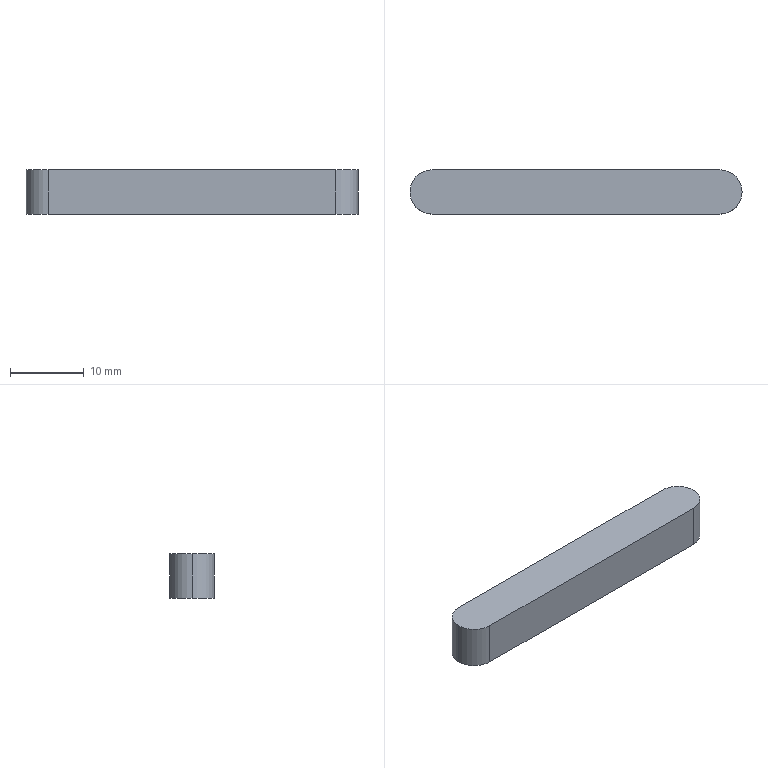Part | STEP file | BPSP-03-008 Flat Key_Default | 1 solid | 8 faces | box 45 x 6 x 6 mm | volume 1574 mm3 | plane 4 | cylinder 4 | commonest cylinder face diameters 6 x4
STEP:
#1=CARTESIAN_POINT('',(0.,0.,0.));
#2=DIRECTION('',(0.,0.,1.));
#3=DIRECTION('',(1.,0.,0.));
#4=AXIS2_PLACEMENT_3D('',#1,#2,#3);
#5=CARTESIAN_POINT('',(19.5,3.,-3.));
#6=VERTEX_POINT('',#5);
#7=CARTESIAN_POINT('',(-19.5,3.,-3.));
#8=VERTEX_POINT('',#7);
#9=CARTESIAN_POINT('',(-22.5,3.,-3.));
#10=DIRECTION('',(-1.,0.,0.));
#11=VECTOR('',#10,1.);
#12=LINE('',#9,#11);
#13=CARTESIAN_POINT('',(-22.5,3.,3.));
#14=DIRECTION('',(0.,-1.,0.));
#15=DIRECTION('',(0.,0.,-1.));
#16=AXIS2_PLACEMENT_3D('',#13,#14,#15);
#17=PLANE('',#16);
#18=CARTESIAN_POINT('',(6.,0.));
#19=DIRECTION('',(0.,-1.));
#20=VECTOR('',#19,1.);
#21=LINE('',#18,#20);
#22=(GEOMETRIC_REPRESENTATION_CONTEXT(2)PARAMETRIC_REPRESENTATION_CONTEXT()REPRESENTATION_CONTEXT('',''));
#23=DEFINITIONAL_REPRESENTATION('',(#21),#22);
#24=PCURVE('',#17,#23);
#25=CARTESIAN_POINT('',(0.,0.,-3.));
#26=DIRECTION('',(0.,0.,1.));
#27=DIRECTION('',(1.,0.,0.));
#28=AXIS2_PLACEMENT_3D('',#25,#26,#27);
#29=PLANE('',#28);
#30=CARTESIAN_POINT('',(-22.5,3.));
#31=DIRECTION('',(-1.,0.));
#32=VECTOR('',#31,1.);
#33=LINE('',#30,#32);
#34=(GEOMETRIC_REPRESENTATION_CONTEXT(2)PARAMETRIC_REPRESENTATION_CONTEXT()REPRESENTATION_CONTEXT('',''));
#35=DEFINITIONAL_REPRESENTATION('',(#33),#34);
#36=PCURVE('',#29,#35);
#37=SURFACE_CURVE('',#12,(#24,#36),.PCURVE_S1.);
#38=EDGE_CURVE('',#6,#8,#37,.T.);
#39=ORIENTED_EDGE('',*,*,#38,.T.);
#40=CARTESIAN_POINT('',(-19.5,3.,3.));
#41=VERTEX_POINT('',#40);
#42=CARTESIAN_POINT('',(-19.5,3.,3.));
#43=DIRECTION('',(0.,0.,1.));
#44=VECTOR('',#43,1.);
#45=LINE('',#42,#44);
#46=CARTESIAN_POINT('',(0.,3.));
#47=DIRECTION('',(-1.,0.));
#48=VECTOR('',#47,1.);
#49=LINE('',#46,#48);
#50=(GEOMETRIC_REPRESENTATION_CONTEXT(2)PARAMETRIC_REPRESENTATION_CONTEXT()REPRESENTATION_CONTEXT('',''));
#51=DEFINITIONAL_REPRESENTATION('',(#49),#50);
#52=PCURVE('',#17,#51);
#53=CARTESIAN_POINT('',(-19.5,0.,3.));
#54=DIRECTION('',(0.,0.,-1.));
#55=DIRECTION('',(-1.,0.,0.));
#56=AXIS2_PLACEMENT_3D('',#53,#54,#55);
#57=CYLINDRICAL_SURFACE('',#56,3.);
#58=CARTESIAN_POINT('',(1.571,0.));
#59=DIRECTION('',(0.,-1.));
#60=VECTOR('',#59,1.);
#61=LINE('',#58,#60);
#62=(GEOMETRIC_REPRESENTATION_CONTEXT(2)PARAMETRIC_REPRESENTATION_CONTEXT()REPRESENTATION_CONTEXT('',''));
#63=DEFINITIONAL_REPRESENTATION('',(#61),#62);
#64=PCURVE('',#57,#63);
#65=SURFACE_CURVE('',#45,(#52,#64),.PCURVE_S1.);
#66=EDGE_CURVE('',#8,#41,#65,.T.);
#67=ORIENTED_EDGE('',*,*,#66,.T.);
#68=CARTESIAN_POINT('',(19.5,3.,3.));
#69=VERTEX_POINT('',#68);
#70=CARTESIAN_POINT('',(-22.5,3.,3.));
#71=DIRECTION('',(-1.,0.,0.));
#72=VECTOR('',#71,1.);
#73=LINE('',#70,#72);
#74=CARTESIAN_POINT('',(0.,0.));
#75=DIRECTION('',(0.,-1.));
#76=VECTOR('',#75,1.);
#77=LINE('',#74,#76);
#78=(GEOMETRIC_REPRESENTATION_CONTEXT(2)PARAMETRIC_REPRESENTATION_CONTEXT()REPRESENTATION_CONTEXT('',''));
#79=DEFINITIONAL_REPRESENTATION('',(#77),#78);
#80=PCURVE('',#17,#79);
#81=CARTESIAN_POINT('',(0.,0.,3.));
#82=DIRECTION('',(0.,0.,1.));
#83=DIRECTION('',(1.,0.,0.));
#84=AXIS2_PLACEMENT_3D('',#81,#82,#83);
#85=PLANE('',#84);
#86=CARTESIAN_POINT('',(-22.5,3.));
#87=DIRECTION('',(-1.,0.));
#88=VECTOR('',#87,1.);
#89=LINE('',#86,#88);
#90=(GEOMETRIC_REPRESENTATION_CONTEXT(2)PARAMETRIC_REPRESENTATION_CONTEXT()REPRESENTATION_CONTEXT('',''));
#91=DEFINITIONAL_REPRESENTATION('',(#89),#90);
#92=PCURVE('',#85,#91);
#93=SURFACE_CURVE('',#73,(#80,#92),.PCURVE_S1.);
#94=EDGE_CURVE('',#69,#41,#93,.T.);
#95=ORIENTED_EDGE('',*,*,#94,.F.);
#96=CARTESIAN_POINT('',(19.5,3.,3.));
#97=DIRECTION('',(0.,0.,-1.));
#98=VECTOR('',#97,1.);
#99=LINE('',#96,#98);
#100=CARTESIAN_POINT('',(0.,42.));
#101=DIRECTION('',(1.,0.));
#102=VECTOR('',#101,1.);
#103=LINE('',#100,#102);
#104=(GEOMETRIC_REPRESENTATION_CONTEXT(2)PARAMETRIC_REPRESENTATION_CONTEXT()REPRESENTATION_CONTEXT('',''));
#105=DEFINITIONAL_REPRESENTATION('',(#103),#104);
#106=PCURVE('',#17,#105);
#107=CARTESIAN_POINT('',(19.5,0.,3.));
#108=DIRECTION('',(0.,0.,-1.));
#109=DIRECTION('',(-1.,0.,0.));
#110=AXIS2_PLACEMENT_3D('',#107,#108,#109);
#111=CYLINDRICAL_SURFACE('',#110,3.);
#112=CARTESIAN_POINT('',(1.571,0.));
#113=DIRECTION('',(0.,1.));
#114=VECTOR('',#113,1.);
#115=LINE('',#112,#114);
#116=(GEOMETRIC_REPRESENTATION_CONTEXT(2)PARAMETRIC_REPRESENTATION_CONTEXT()REPRESENTATION_CONTEXT('',''));
#117=DEFINITIONAL_REPRESENTATION('',(#115),#116);
#118=PCURVE('',#111,#117);
#119=SURFACE_CURVE('',#99,(#106,#118),.PCURVE_S1.);
#120=EDGE_CURVE('',#69,#6,#119,.T.);
#121=ORIENTED_EDGE('',*,*,#120,.T.);
#122=EDGE_LOOP('',(#39,#67,#95,#121));
#123=FACE_BOUND('',#122,.T.);
#124=ADVANCED_FACE('',(#123),#17,.F.);
#125=CARTESIAN_POINT('',(-19.5,-3.,3.));
#126=VERTEX_POINT('',#125);
#127=CARTESIAN_POINT('',(19.5,-3.,3.));
#128=VERTEX_POINT('',#127);
#129=CARTESIAN_POINT('',(-22.5,-3.,3.));
#130=DIRECTION('',(1.,0.,0.));
#131=VECTOR('',#130,1.);
#132=LINE('',#129,#131);
#133=CARTESIAN_POINT('',(-22.5,-3.,3.));
#134=DIRECTION('',(0.,1.,0.));
#135=DIRECTION('',(0.,0.,1.));
#136=AXIS2_PLACEMENT_3D('',#133,#134,#135);
#137=PLANE('',#136);
#138=CARTESIAN_POINT('',(0.,0.));
#139=DIRECTION('',(0.,1.));
#140=VECTOR('',#139,1.);
#141=LINE('',#138,#140);
#142=(GEOMETRIC_REPRESENTATION_CONTEXT(2)PARAMETRIC_REPRESENTATION_CONTEXT()REPRESENTATION_CONTEXT('',''));
#143=DEFINITIONAL_REPRESENTATION('',(#141),#142);
#144=PCURVE('',#137,#143);
#145=CARTESIAN_POINT('',(-22.5,-3.));
#146=DIRECTION('',(1.,0.));
#147=VECTOR('',#146,1.);
#148=LINE('',#145,#147);
#149=(GEOMETRIC_REPRESENTATION_CONTEXT(2)PARAMETRIC_REPRESENTATION_CONTEXT()REPRESENTATION_CONTEXT('',''));
#150=DEFINITIONAL_REPRESENTATION('',(#148),#149);
#151=PCURVE('',#85,#150);
#152=SURFACE_CURVE('',#132,(#144,#151),.PCURVE_S1.);
#153=EDGE_CURVE('',#126,#128,#152,.T.);
#154=ORIENTED_EDGE('',*,*,#153,.F.);
#155=CARTESIAN_POINT('',(-19.5,-3.,-3.));
#156=VERTEX_POINT('',#155);
#157=CARTESIAN_POINT('',(-19.5,-3.,3.));
#158=DIRECTION('',(0.,0.,-1.));
#159=VECTOR('',#158,1.);
#160=LINE('',#157,#159);
#161=CARTESIAN_POINT('',(0.,3.));
#162=DIRECTION('',(-1.,0.));
#163=VECTOR('',#162,1.);
#164=LINE('',#161,#163);
#165=(GEOMETRIC_REPRESENTATION_CONTEXT(2)PARAMETRIC_REPRESENTATION_CONTEXT()REPRESENTATION_CONTEXT('',''));
#166=DEFINITIONAL_REPRESENTATION('',(#164),#165);
#167=PCURVE('',#137,#166);
#168=CARTESIAN_POINT('',(-19.5,0.,3.));
#169=DIRECTION('',(0.,0.,-1.));
#170=DIRECTION('',(-1.,0.,0.));
#171=AXIS2_PLACEMENT_3D('',#168,#169,#170);
#172=CYLINDRICAL_SURFACE('',#171,3.);
#173=CARTESIAN_POINT('',(4.712,0.));
#174=DIRECTION('',(0.,1.));
#175=VECTOR('',#174,1.);
#176=LINE('',#173,#175);
#177=(GEOMETRIC_REPRESENTATION_CONTEXT(2)PARAMETRIC_REPRESENTATION_CONTEXT()REPRESENTATION_CONTEXT('',''));
#178=DEFINITIONAL_REPRESENTATION('',(#176),#177);
#179=PCURVE('',#172,#178);
#180=SURFACE_CURVE('',#160,(#167,#179),.PCURVE_S1.);
#181=EDGE_CURVE('',#126,#156,#180,.T.);
#182=ORIENTED_EDGE('',*,*,#181,.T.);
#183=CARTESIAN_POINT('',(19.5,-3.,-3.));
#184=VERTEX_POINT('',#183);
#185=CARTESIAN_POINT('',(-22.5,-3.,-3.));
#186=DIRECTION('',(1.,0.,0.));
#187=VECTOR('',#186,1.);
#188=LINE('',#185,#187);
#189=CARTESIAN_POINT('',(-6.,0.));
#190=DIRECTION('',(0.,1.));
#191=VECTOR('',#190,1.);
#192=LINE('',#189,#191);
#193=(GEOMETRIC_REPRESENTATION_CONTEXT(2)PARAMETRIC_REPRESENTATION_CONTEXT()REPRESENTATION_CONTEXT('',''));
#194=DEFINITIONAL_REPRESENTATION('',(#192),#193);
#195=PCURVE('',#137,#194);
#196=CARTESIAN_POINT('',(-22.5,-3.));
#197=DIRECTION('',(1.,0.));
#198=VECTOR('',#197,1.);
#199=LINE('',#196,#198);
#200=(GEOMETRIC_REPRESENTATION_CONTEXT(2)PARAMETRIC_REPRESENTATION_CONTEXT()REPRESENTATION_CONTEXT('',''));
#201=DEFINITIONAL_REPRESENTATION('',(#199),#200);
#202=PCURVE('',#29,#201);
#203=SURFACE_CURVE('',#188,(#195,#202),.PCURVE_S1.);
#204=EDGE_CURVE('',#156,#184,#203,.T.);
#205=ORIENTED_EDGE('',*,*,#204,.T.);
#206=CARTESIAN_POINT('',(19.5,-3.,3.));
#207=DIRECTION('',(0.,0.,1.));
#208=VECTOR('',#207,1.);
#209=LINE('',#206,#208);
#210=CARTESIAN_POINT('',(0.,42.));
#211=DIRECTION('',(1.,0.));
#212=VECTOR('',#211,1.);
#213=LINE('',#210,#212);
#214=(GEOMETRIC_REPRESENTATION_CONTEXT(2)PARAMETRIC_REPRESENTATION_CONTEXT()REPRESENTATION_CONTEXT('',''));
#215=DEFINITIONAL_REPRESENTATION('',(#213),#214);
#216=PCURVE('',#137,#215);
#217=CARTESIAN_POINT('',(19.5,0.,3.));
#218=DIRECTION('',(0.,0.,-1.));
#219=DIRECTION('',(-1.,0.,0.));
#220=AXIS2_PLACEMENT_3D('',#217,#218,#219);
#221=CYLINDRICAL_SURFACE('',#220,3.);
#222=CARTESIAN_POINT('',(4.712,0.));
#223=DIRECTION('',(0.,-1.));
#224=VECTOR('',#223,1.);
#225=LINE('',#222,#224);
#226=(GEOMETRIC_REPRESENTATION_CONTEXT(2)PARAMETRIC_REPRESENTATION_CONTEXT()REPRESENTATION_CONTEXT('',''));
#227=DEFINITIONAL_REPRESENTATION('',(#225),#226);
#228=PCURVE('',#221,#227);
#229=SURFACE_CURVE('',#209,(#216,#228),.PCURVE_S1.);
#230=EDGE_CURVE('',#184,#128,#229,.T.);
#231=ORIENTED_EDGE('',*,*,#230,.T.);
#232=EDGE_LOOP('',(#154,#182,#205,#231));
#233=FACE_BOUND('',#232,.T.);
#234=ADVANCED_FACE('',(#233),#137,.F.);
#235=CARTESIAN_POINT('',(-22.5,0.,3.));
#236=VERTEX_POINT('',#235);
#237=CARTESIAN_POINT('',(-19.5,0.,3.));
#238=DIRECTION('',(0.,0.,1.));
#239=DIRECTION('',(1.,0.,0.));
#240=AXIS2_PLACEMENT_3D('',#237,#238,#239);
#241=CIRCLE('',#240,3.);
#242=CARTESIAN_POINT('',(-19.5,0.));
#243=DIRECTION('',(1.,0.));
#244=AXIS2_PLACEMENT_2D('',#242,#243);
#245=CIRCLE('',#244,3.);
#246=(GEOMETRIC_REPRESENTATION_CONTEXT(2)PARAMETRIC_REPRESENTATION_CONTEXT()REPRESENTATION_CONTEXT('',''));
#247=DEFINITIONAL_REPRESENTATION('',(#245),#246);
#248=PCURVE('',#85,#247);
#249=CARTESIAN_POINT('',(3.142,0.));
#250=DIRECTION('',(-1.,0.));
#251=VECTOR('',#250,1.);
#252=LINE('',#249,#251);
#253=(GEOMETRIC_REPRESENTATION_CONTEXT(2)PARAMETRIC_REPRESENTATION_CONTEXT()REPRESENTATION_CONTEXT('',''));
#254=DEFINITIONAL_REPRESENTATION('',(#252),#253);
#255=PCURVE('',#57,#254);
#256=SURFACE_CURVE('',#241,(#248,#255),.PCURVE_S1.);
#257=EDGE_CURVE('',#41,#236,#256,.T.);
#258=ORIENTED_EDGE('',*,*,#257,.T.);
#259=CARTESIAN_POINT('',(-19.5,0.,3.));
#260=DIRECTION('',(0.,0.,1.));
#261=DIRECTION('',(1.,0.,0.));
#262=AXIS2_PLACEMENT_3D('',#259,#260,#261);
#263=CIRCLE('',#262,3.);
#264=CARTESIAN_POINT('',(-19.5,0.));
#265=DIRECTION('',(1.,0.));
#266=AXIS2_PLACEMENT_2D('',#264,#265);
#267=CIRCLE('',#266,3.);
#268=(GEOMETRIC_REPRESENTATION_CONTEXT(2)PARAMETRIC_REPRESENTATION_CONTEXT()REPRESENTATION_CONTEXT('',''));
#269=DEFINITIONAL_REPRESENTATION('',(#267),#268);
#270=PCURVE('',#85,#269);
#271=CARTESIAN_POINT('',(9.425,0.));
#272=DIRECTION('',(-1.,0.));
#273=VECTOR('',#272,1.);
#274=LINE('',#271,#273);
#275=(GEOMETRIC_REPRESENTATION_CONTEXT(2)PARAMETRIC_REPRESENTATION_CONTEXT()REPRESENTATION_CONTEXT('',''));
#276=DEFINITIONAL_REPRESENTATION('',(#274),#275);
#277=PCURVE('',#172,#276);
#278=SURFACE_CURVE('',#263,(#270,#277),.PCURVE_S1.);
#279=EDGE_CURVE('',#236,#126,#278,.T.);
#280=ORIENTED_EDGE('',*,*,#279,.T.);
#281=ORIENTED_EDGE('',*,*,#153,.T.);
#282=CARTESIAN_POINT('',(22.5,0.,3.));
#283=VERTEX_POINT('',#282);
#284=CARTESIAN_POINT('',(19.5,0.,3.));
#285=DIRECTION('',(0.,0.,1.));
#286=DIRECTION('',(1.,0.,0.));
#287=AXIS2_PLACEMENT_3D('',#284,#285,#286);
#288=CIRCLE('',#287,3.);
#289=CARTESIAN_POINT('',(19.5,0.));
#290=DIRECTION('',(1.,0.));
#291=AXIS2_PLACEMENT_2D('',#289,#290);
#292=CIRCLE('',#291,3.);
#293=(GEOMETRIC_REPRESENTATION_CONTEXT(2)PARAMETRIC_REPRESENTATION_CONTEXT()REPRESENTATION_CONTEXT('',''));
#294=DEFINITIONAL_REPRESENTATION('',(#292),#293);
#295=PCURVE('',#85,#294);
#296=CARTESIAN_POINT('',(9.425,0.));
#297=DIRECTION('',(-1.,0.));
#298=VECTOR('',#297,1.);
#299=LINE('',#296,#298);
#300=(GEOMETRIC_REPRESENTATION_CONTEXT(2)PARAMETRIC_REPRESENTATION_CONTEXT()REPRESENTATION_CONTEXT('',''));
#301=DEFINITIONAL_REPRESENTATION('',(#299),#300);
#302=PCURVE('',#221,#301);
#303=SURFACE_CURVE('',#288,(#295,#302),.PCURVE_S1.);
#304=EDGE_CURVE('',#128,#283,#303,.T.);
#305=ORIENTED_EDGE('',*,*,#304,.T.);
#306=CARTESIAN_POINT('',(19.5,0.,3.));
#307=DIRECTION('',(0.,0.,1.));
#308=DIRECTION('',(1.,0.,0.));
#309=AXIS2_PLACEMENT_3D('',#306,#307,#308);
#310=CIRCLE('',#309,3.);
#311=CARTESIAN_POINT('',(19.5,0.));
#312=DIRECTION('',(1.,0.));
#313=AXIS2_PLACEMENT_2D('',#311,#312);
#314=CIRCLE('',#313,3.);
#315=(GEOMETRIC_REPRESENTATION_CONTEXT(2)PARAMETRIC_REPRESENTATION_CONTEXT()REPRESENTATION_CONTEXT('',''));
#316=DEFINITIONAL_REPRESENTATION('',(#314),#315);
#317=PCURVE('',#85,#316);
#318=CARTESIAN_POINT('',(3.142,0.));
#319=DIRECTION('',(-1.,0.));
#320=VECTOR('',#319,1.);
#321=LINE('',#318,#320);
#322=(GEOMETRIC_REPRESENTATION_CONTEXT(2)PARAMETRIC_REPRESENTATION_CONTEXT()REPRESENTATION_CONTEXT('',''));
#323=DEFINITIONAL_REPRESENTATION('',(#321),#322);
#324=PCURVE('',#111,#323);
#325=SURFACE_CURVE('',#310,(#317,#324),.PCURVE_S1.);
#326=EDGE_CURVE('',#283,#69,#325,.T.);
#327=ORIENTED_EDGE('',*,*,#326,.T.);
#328=ORIENTED_EDGE('',*,*,#94,.T.);
#329=EDGE_LOOP('',(#258,#280,#281,#305,#327,#328));
#330=FACE_BOUND('',#329,.T.);
#331=ADVANCED_FACE('',(#330),#85,.T.);
#332=ORIENTED_EDGE('',*,*,#204,.F.);
#333=CARTESIAN_POINT('',(-22.5,0.,-3.));
#334=VERTEX_POINT('',#333);
#335=CARTESIAN_POINT('',(-19.5,0.,-3.));
#336=DIRECTION('',(0.,0.,-1.));
#337=DIRECTION('',(1.,0.,0.));
#338=AXIS2_PLACEMENT_3D('',#335,#336,#337);
#339=CIRCLE('',#338,3.);
#340=CARTESIAN_POINT('',(-16.5,0.));
#341=CARTESIAN_POINT('',(-16.5,-5.196));
#342=CARTESIAN_POINT('',(-21.,-2.598));
#343=CARTESIAN_POINT('',(-25.5,0.));
#344=CARTESIAN_POINT('',(-21.,2.598));
#345=CARTESIAN_POINT('',(-16.5,5.196));
#346=CARTESIAN_POINT('',(-16.5,0.));
#347=(BOUNDED_CURVE()B_SPLINE_CURVE(2,(#340,#341,#342,#343,#344,#345,#346),.UNSPECIFIED.,.T.,.F.)B_SPLINE_CURVE_WITH_KNOTS((1,2,2,2,2,1),(-2.094,0.,2.094,4.189,6.283,8.378),.UNSPECIFIED.)CURVE()GEOMETRIC_REPRESENTATION_ITEM()RATIONAL_B_SPLINE_CURVE((1.,0.5,1.,0.5,1.,0.5,1.))REPRESENTATION_ITEM(''));
#348=(GEOMETRIC_REPRESENTATION_CONTEXT(2)PARAMETRIC_REPRESENTATION_CONTEXT()REPRESENTATION_CONTEXT('',''));
#349=DEFINITIONAL_REPRESENTATION('',(#347),#348);
#350=PCURVE('',#29,#349);
#351=CARTESIAN_POINT('',(3.142,6.));
#352=DIRECTION('',(1.,0.));
#353=VECTOR('',#352,1.);
#354=LINE('',#351,#353);
#355=(GEOMETRIC_REPRESENTATION_CONTEXT(2)PARAMETRIC_REPRESENTATION_CONTEXT()REPRESENTATION_CONTEXT('',''));
#356=DEFINITIONAL_REPRESENTATION('',(#354),#355);
#357=PCURVE('',#172,#356);
#358=SURFACE_CURVE('',#339,(#350,#357),.PCURVE_S1.);
#359=EDGE_CURVE('',#156,#334,#358,.T.);
#360=ORIENTED_EDGE('',*,*,#359,.T.);
#361=CARTESIAN_POINT('',(-19.5,0.,-3.));
#362=DIRECTION('',(0.,0.,-1.));
#363=DIRECTION('',(1.,0.,0.));
#364=AXIS2_PLACEMENT_3D('',#361,#362,#363);
#365=CIRCLE('',#364,3.);
#366=CARTESIAN_POINT('',(-16.5,0.));
#367=CARTESIAN_POINT('',(-16.5,-5.196));
#368=CARTESIAN_POINT('',(-21.,-2.598));
#369=CARTESIAN_POINT('',(-25.5,0.));
#370=CARTESIAN_POINT('',(-21.,2.598));
#371=CARTESIAN_POINT('',(-16.5,5.196));
#372=CARTESIAN_POINT('',(-16.5,0.));
#373=(BOUNDED_CURVE()B_SPLINE_CURVE(2,(#366,#367,#368,#369,#370,#371,#372),.UNSPECIFIED.,.T.,.F.)B_SPLINE_CURVE_WITH_KNOTS((1,2,2,2,2,1),(-2.094,0.,2.094,4.189,6.283,8.378),.UNSPECIFIED.)CURVE()GEOMETRIC_REPRESENTATION_ITEM()RATIONAL_B_SPLINE_CURVE((1.,0.5,1.,0.5,1.,0.5,1.))REPRESENTATION_ITEM(''));
#374=(GEOMETRIC_REPRESENTATION_CONTEXT(2)PARAMETRIC_REPRESENTATION_CONTEXT()REPRESENTATION_CONTEXT('',''));
#375=DEFINITIONAL_REPRESENTATION('',(#373),#374);
#376=PCURVE('',#29,#375);
#377=CARTESIAN_POINT('',(-3.142,6.));
#378=DIRECTION('',(1.,0.));
#379=VECTOR('',#378,1.);
#380=LINE('',#377,#379);
#381=(GEOMETRIC_REPRESENTATION_CONTEXT(2)PARAMETRIC_REPRESENTATION_CONTEXT()REPRESENTATION_CONTEXT('',''));
#382=DEFINITIONAL_REPRESENTATION('',(#380),#381);
#383=PCURVE('',#57,#382);
#384=SURFACE_CURVE('',#365,(#376,#383),.PCURVE_S1.);
#385=EDGE_CURVE('',#334,#8,#384,.T.);
#386=ORIENTED_EDGE('',*,*,#385,.T.);
#387=ORIENTED_EDGE('',*,*,#38,.F.);
#388=CARTESIAN_POINT('',(22.5,0.,-3.));
#389=VERTEX_POINT('',#388);
#390=CARTESIAN_POINT('',(19.5,0.,-3.));
#391=DIRECTION('',(0.,0.,-1.));
#392=DIRECTION('',(1.,0.,0.));
#393=AXIS2_PLACEMENT_3D('',#390,#391,#392);
#394=CIRCLE('',#393,3.);
#395=CARTESIAN_POINT('',(22.5,0.));
#396=CARTESIAN_POINT('',(22.5,-5.196));
#397=CARTESIAN_POINT('',(18.,-2.598));
#398=CARTESIAN_POINT('',(13.5,0.));
#399=CARTESIAN_POINT('',(18.,2.598));
#400=CARTESIAN_POINT('',(22.5,5.196));
#401=CARTESIAN_POINT('',(22.5,0.));
#402=(BOUNDED_CURVE()B_SPLINE_CURVE(2,(#395,#396,#397,#398,#399,#400,#401),.UNSPECIFIED.,.T.,.F.)B_SPLINE_CURVE_WITH_KNOTS((1,2,2,2,2,1),(-2.094,0.,2.094,4.189,6.283,8.378),.UNSPECIFIED.)CURVE()GEOMETRIC_REPRESENTATION_ITEM()RATIONAL_B_SPLINE_CURVE((1.,0.5,1.,0.5,1.,0.5,1.))REPRESENTATION_ITEM(''));
#403=(GEOMETRIC_REPRESENTATION_CONTEXT(2)PARAMETRIC_REPRESENTATION_CONTEXT()REPRESENTATION_CONTEXT('',''));
#404=DEFINITIONAL_REPRESENTATION('',(#402),#403);
#405=PCURVE('',#29,#404);
#406=CARTESIAN_POINT('',(-3.142,6.));
#407=DIRECTION('',(1.,0.));
#408=VECTOR('',#407,1.);
#409=LINE('',#406,#408);
#410=(GEOMETRIC_REPRESENTATION_CONTEXT(2)PARAMETRIC_REPRESENTATION_CONTEXT()REPRESENTATION_CONTEXT('',''));
#411=DEFINITIONAL_REPRESENTATION('',(#409),#410);
#412=PCURVE('',#111,#411);
#413=SURFACE_CURVE('',#394,(#405,#412),.PCURVE_S1.);
#414=EDGE_CURVE('',#6,#389,#413,.T.);
#415=ORIENTED_EDGE('',*,*,#414,.T.);
#416=CARTESIAN_POINT('',(19.5,0.,-3.));
#417=DIRECTION('',(0.,0.,-1.));
#418=DIRECTION('',(1.,0.,0.));
#419=AXIS2_PLACEMENT_3D('',#416,#417,#418);
#420=CIRCLE('',#419,3.);
#421=CARTESIAN_POINT('',(22.5,0.));
#422=CARTESIAN_POINT('',(22.5,-5.196));
#423=CARTESIAN_POINT('',(18.,-2.598));
#424=CARTESIAN_POINT('',(13.5,0.));
#425=CARTESIAN_POINT('',(18.,2.598));
#426=CARTESIAN_POINT('',(22.5,5.196));
#427=CARTESIAN_POINT('',(22.5,0.));
#428=(BOUNDED_CURVE()B_SPLINE_CURVE(2,(#421,#422,#423,#424,#425,#426,#427),.UNSPECIFIED.,.T.,.F.)B_SPLINE_CURVE_WITH_KNOTS((1,2,2,2,2,1),(-2.094,0.,2.094,4.189,6.283,8.378),.UNSPECIFIED.)CURVE()GEOMETRIC_REPRESENTATION_ITEM()RATIONAL_B_SPLINE_CURVE((1.,0.5,1.,0.5,1.,0.5,1.))REPRESENTATION_ITEM(''));
#429=(GEOMETRIC_REPRESENTATION_CONTEXT(2)PARAMETRIC_REPRESENTATION_CONTEXT()REPRESENTATION_CONTEXT('',''));
#430=DEFINITIONAL_REPRESENTATION('',(#428),#429);
#431=PCURVE('',#29,#430);
#432=CARTESIAN_POINT('',(3.142,6.));
#433=DIRECTION('',(1.,0.));
#434=VECTOR('',#433,1.);
#435=LINE('',#432,#434);
#436=(GEOMETRIC_REPRESENTATION_CONTEXT(2)PARAMETRIC_REPRESENTATION_CONTEXT()REPRESENTATION_CONTEXT('',''));
#437=DEFINITIONAL_REPRESENTATION('',(#435),#436);
#438=PCURVE('',#221,#437);
#439=SURFACE_CURVE('',#420,(#431,#438),.PCURVE_S1.);
#440=EDGE_CURVE('',#389,#184,#439,.T.);
#441=ORIENTED_EDGE('',*,*,#440,.T.);
#442=EDGE_LOOP('',(#332,#360,#386,#387,#415,#441));
#443=FACE_BOUND('',#442,.T.);
#444=ADVANCED_FACE('',(#443),#29,.F.);
#445=CARTESIAN_POINT('',(-22.5,0.,3.));
#446=DIRECTION('',(0.,0.,-1.));
#447=VECTOR('',#446,1.);
#448=LINE('',#445,#447);
#449=CARTESIAN_POINT('',(0.,0.));
#450=DIRECTION('',(0.,1.));
#451=VECTOR('',#450,1.);
#452=LINE('',#449,#451);
#453=(GEOMETRIC_REPRESENTATION_CONTEXT(2)PARAMETRIC_REPRESENTATION_CONTEXT()REPRESENTATION_CONTEXT('',''));
#454=DEFINITIONAL_REPRESENTATION('',(#452),#453);
#455=PCURVE('',#57,#454);
#456=CARTESIAN_POINT('',(6.283,0.));
#457=DIRECTION('',(0.,1.));
#458=VECTOR('',#457,1.);
#459=LINE('',#456,#458);
#460=(GEOMETRIC_REPRESENTATION_CONTEXT(2)PARAMETRIC_REPRESENTATION_CONTEXT()REPRESENTATION_CONTEXT('',''));
#461=DEFINITIONAL_REPRESENTATION('',(#459),#460);
#462=PCURVE('',#172,#461);
#463=SURFACE_CURVE('',#448,(#455,#462),.PCURVE_S1.);
#464=EDGE_CURVE('',#236,#334,#463,.T.);
#465=ORIENTED_EDGE('',*,*,#464,.F.);
#466=ORIENTED_EDGE('',*,*,#257,.F.);
#467=ORIENTED_EDGE('',*,*,#66,.F.);
#468=ORIENTED_EDGE('',*,*,#385,.F.);
#469=EDGE_LOOP('',(#465,#466,#467,#468));
#470=FACE_BOUND('',#469,.T.);
#471=ADVANCED_FACE('',(#470),#57,.T.);
#472=ORIENTED_EDGE('',*,*,#279,.F.);
#473=ORIENTED_EDGE('',*,*,#464,.T.);
#474=ORIENTED_EDGE('',*,*,#359,.F.);
#475=ORIENTED_EDGE('',*,*,#181,.F.);
#476=EDGE_LOOP('',(#472,#473,#474,#475));
#477=FACE_BOUND('',#476,.T.);
#478=ADVANCED_FACE('',(#477),#172,.T.);
#479=ORIENTED_EDGE('',*,*,#120,.F.);
#480=ORIENTED_EDGE('',*,*,#326,.F.);
#481=CARTESIAN_POINT('',(22.5,0.,3.));
#482=DIRECTION('',(0.,0.,1.));
#483=VECTOR('',#482,1.);
#484=LINE('',#481,#483);
#485=CARTESIAN_POINT('',(3.142,0.));
#486=DIRECTION('',(0.,-1.));
#487=VECTOR('',#486,1.);
#488=LINE('',#485,#487);
#489=(GEOMETRIC_REPRESENTATION_CONTEXT(2)PARAMETRIC_REPRESENTATION_CONTEXT()REPRESENTATION_CONTEXT('',''));
#490=DEFINITIONAL_REPRESENTATION('',(#488),#489);
#491=PCURVE('',#111,#490);
#492=CARTESIAN_POINT('',(3.142,0.));
#493=DIRECTION('',(0.,-1.));
#494=VECTOR('',#493,1.);
#495=LINE('',#492,#494);
#496=(GEOMETRIC_REPRESENTATION_CONTEXT(2)PARAMETRIC_REPRESENTATION_CONTEXT()REPRESENTATION_CONTEXT('',''));
#497=DEFINITIONAL_REPRESENTATION('',(#495),#496);
#498=PCURVE('',#221,#497);
#499=SURFACE_CURVE('',#484,(#491,#498),.PCURVE_S1.);
#500=EDGE_CURVE('',#389,#283,#499,.T.);
#501=ORIENTED_EDGE('',*,*,#500,.F.);
#502=ORIENTED_EDGE('',*,*,#414,.F.);
#503=EDGE_LOOP('',(#479,#480,#501,#502));
#504=FACE_BOUND('',#503,.T.);
#505=ADVANCED_FACE('',(#504),#111,.T.);
#506=ORIENTED_EDGE('',*,*,#304,.F.);
#507=ORIENTED_EDGE('',*,*,#230,.F.);
#508=ORIENTED_EDGE('',*,*,#440,.F.);
#509=ORIENTED_EDGE('',*,*,#500,.T.);
#510=EDGE_LOOP('',(#506,#507,#508,#509));
#511=FACE_BOUND('',#510,.T.);
#512=ADVANCED_FACE('',(#511),#221,.T.);
#513=CLOSED_SHELL('',(#124,#234,#331,#444,#471,#478,#505,#512));
#514=MANIFOLD_SOLID_BREP('',#513);
#515=(LENGTH_UNIT()NAMED_UNIT(*)SI_UNIT(.MILLI.,.METRE.));
#516=UNCERTAINTY_MEASURE_WITH_UNIT(LENGTH_MEASURE(0.0000001),#515,'','');
#517=(NAMED_UNIT(*)PLANE_ANGLE_UNIT()SI_UNIT($,.RADIAN.));
#518=(NAMED_UNIT(*)SI_UNIT($,.STERADIAN.)SOLID_ANGLE_UNIT());
#519=(GEOMETRIC_REPRESENTATION_CONTEXT(3)GLOBAL_UNCERTAINTY_ASSIGNED_CONTEXT((#516))GLOBAL_UNIT_ASSIGNED_CONTEXT((#515,#517,#518))REPRESENTATION_CONTEXT('',''));
#520=ADVANCED_BREP_SHAPE_REPRESENTATION('',(#4,#514),#519);